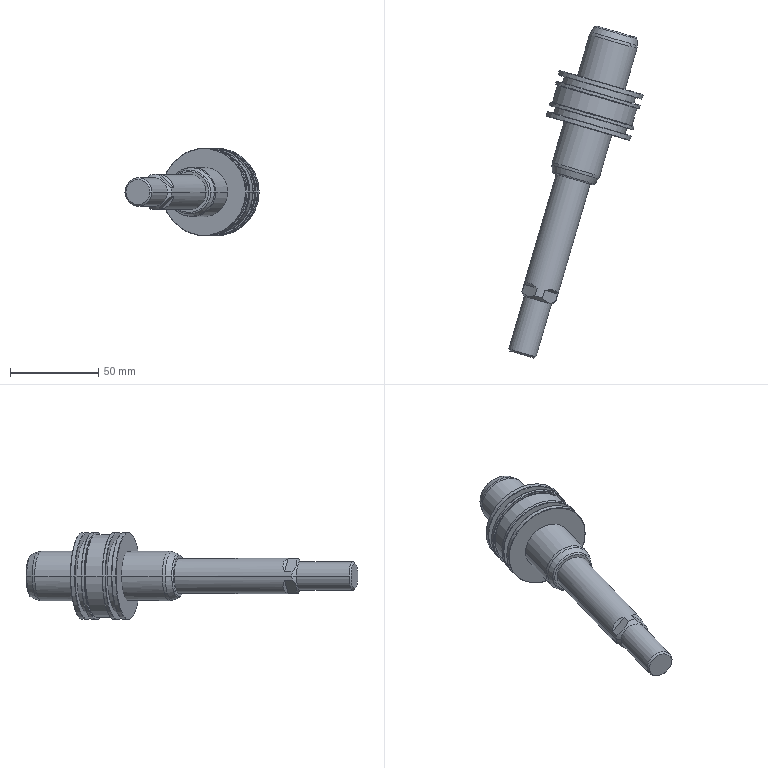Part | SolidWorks | features BaseBody 1 | 1 solid | 84 faces | box 76.059 x 188.139 x 49.5 mm | volume 95194 mm3 | cone 28 | cylinder 24 | plane 20 | spline 12 | commonest cylinder face diameters 49.5 x8 28 x4 42 x4 16 x2 19 x2 20 x2